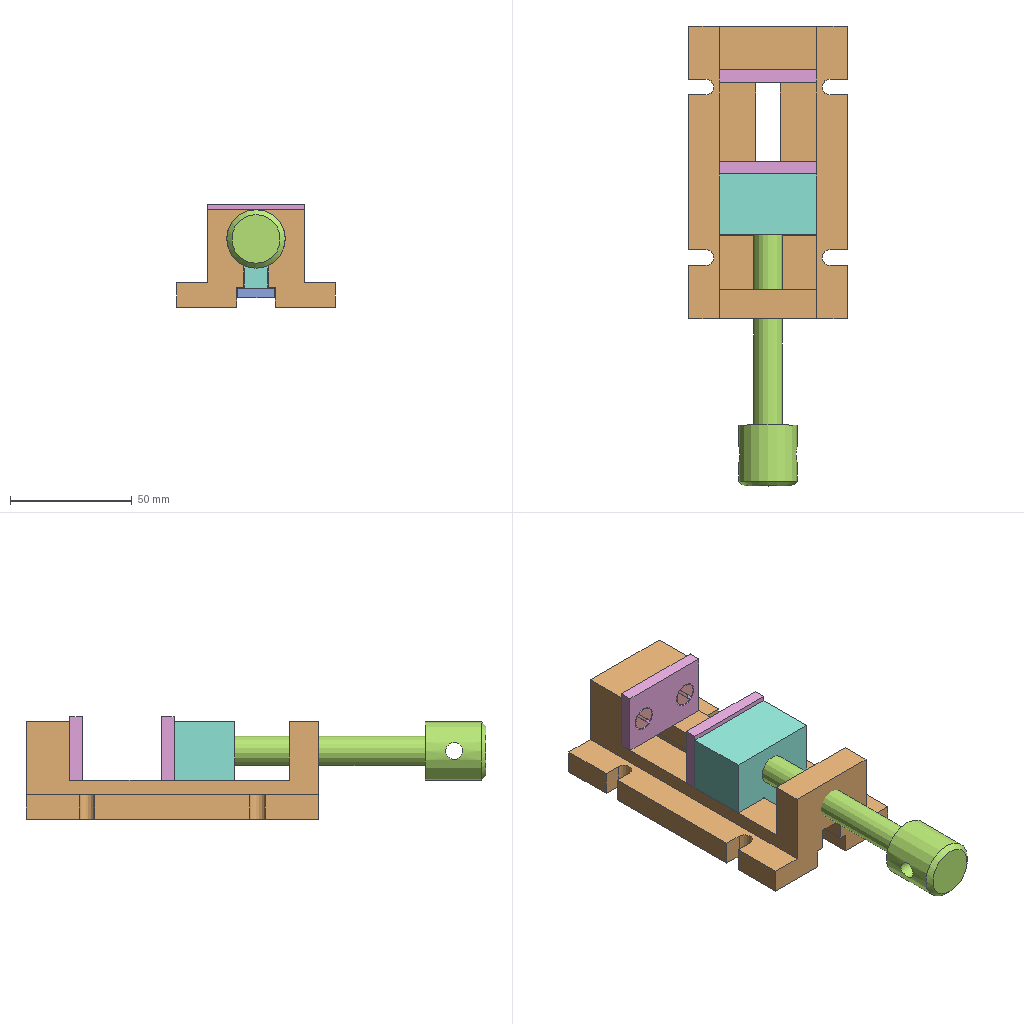Assembly | NX | 6 different items | 11 placed | box 65 x 189 x 42 mm
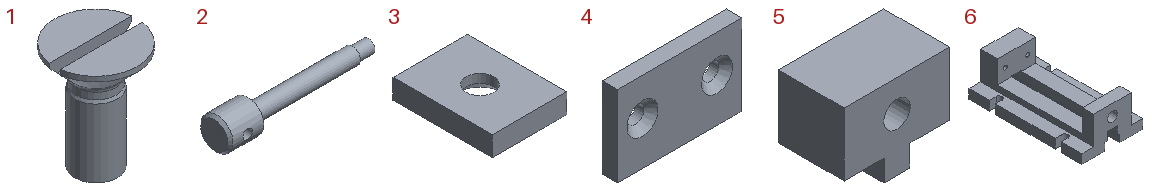Parts list (item | quantity | size | volume | features):
1 | x5 | 9.222 x 9.3 x 12 mm | 279.35 mm3 | features DATUM_CSYS 2, SKETCH 2, EXTRUDE 1, LINE 1, META 1, SWP104 1, SYMBOLIC_THREAD 1, THREADS 1
2 | x1 | 115 x 24 x 24 mm | 19981 mm3 | features CYLINDER 3, CHAMFER 1, DATUM_CSYS 1, HOLE PACKAGE 1, POINT 1, SIMPLE HOLE 1, SYMBOLIC_THREAD 1
3 | x1 | 15 x 20 x 4 mm | 1049 mm3 | features DATUM_CSYS 2, CSUNK_HOLE 1, EXTRUDE 1, HOLE PACKAGE 1, SKETCH 1
4 | x2 | 40 x 5 x 26 mm | 4851 mm3 | features DATUM_CSYS 3, CSUNK_HOLE 2, SKETCH 2, EXTRUDE 1, HOLE PACKAGE 1
5 | x1 | 40 x 25 x 32.2 mm | 24398 mm3 | features DATUM_CSYS 5, SIMPLE HOLE 4, SKETCH 4, HOLE PACKAGE 3, SYMBOLIC_THREAD 3, EXTRUDE 1
6 | x1 | 65 x 120 x 40 mm | 106229 mm3 | features DATUM_CSYS 8, SKETCH 7, EXTRUDE 5, SIMPLE HOLE 5, HOLE PACKAGE 3, SYMBOLIC_THREAD 3
Mates (type | each side: item.copy, entity, surface, feature):
Fix | 6.1 component
Concentric | 4.1 edge | 6.1 edge | 2 times
Center22 | 5.1 face plane Extrude(8) | 5.1 face plane Extrude(8) | 6.1 face plane Extrude(9) | 6.1 face plane Extrude(9)
Touch | 5.1 face plane Extrude(8) | 6.1 face plane Extrude(10)
Concentric | 4.1 edge | 5.1 edge | 2 times
Concentric | 3.1 edge | 5.1 edge
Concentric | 2.1 edge | 5.1 edge
Touch | 1.1 face cylinder Revolve(4) | 3.1 face cylinder Ø5.5 Countersunk Hole(9)
Angle | 1.1 face plane Extrude(5) | 3.1 face plane Extrude(8)
Touch | 1.1 face cylinder Revolve(4) | 4.1 face cylinder Ø5.5 Countersunk Hole(9) | 4 times
Angle | 1.1 face plane Extrude(5) | 4.1 face plane Extrude(8) | 4 times